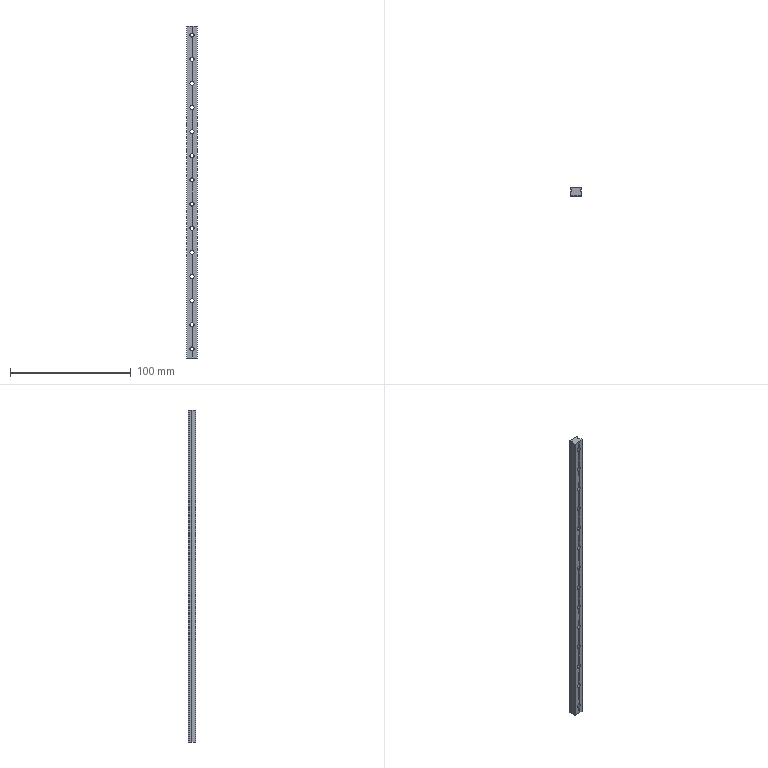Part | STEP file | MGN9CR275 | 1 solid | 101 faces | box 9 x 6.5 x 275 mm | volume 13419 mm3 | cylinder 74 | plane 27 | commonest cylinder face diameters 6 x28 3.4 x22 0.6 x15 3.5 x6 2 x3